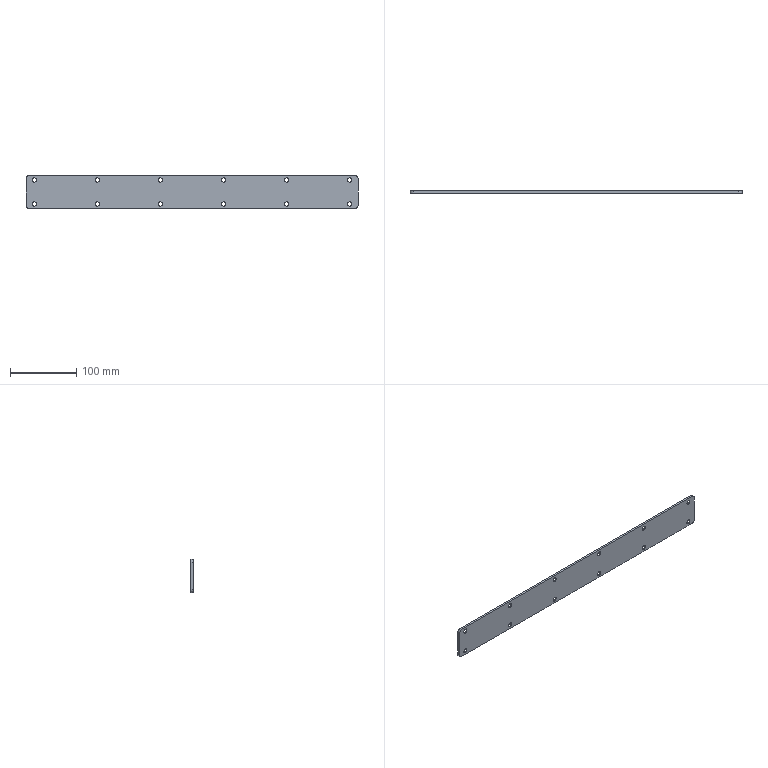Part | STEP file | BT2022003-10 Liner plate | 1 solid | 58 faces | box 500 x 4 x 50 mm | volume 96702 mm3 | cylinder 28 | cone 24 | plane 6 | commonest cylinder face diameters 6.6 x24 10 x4